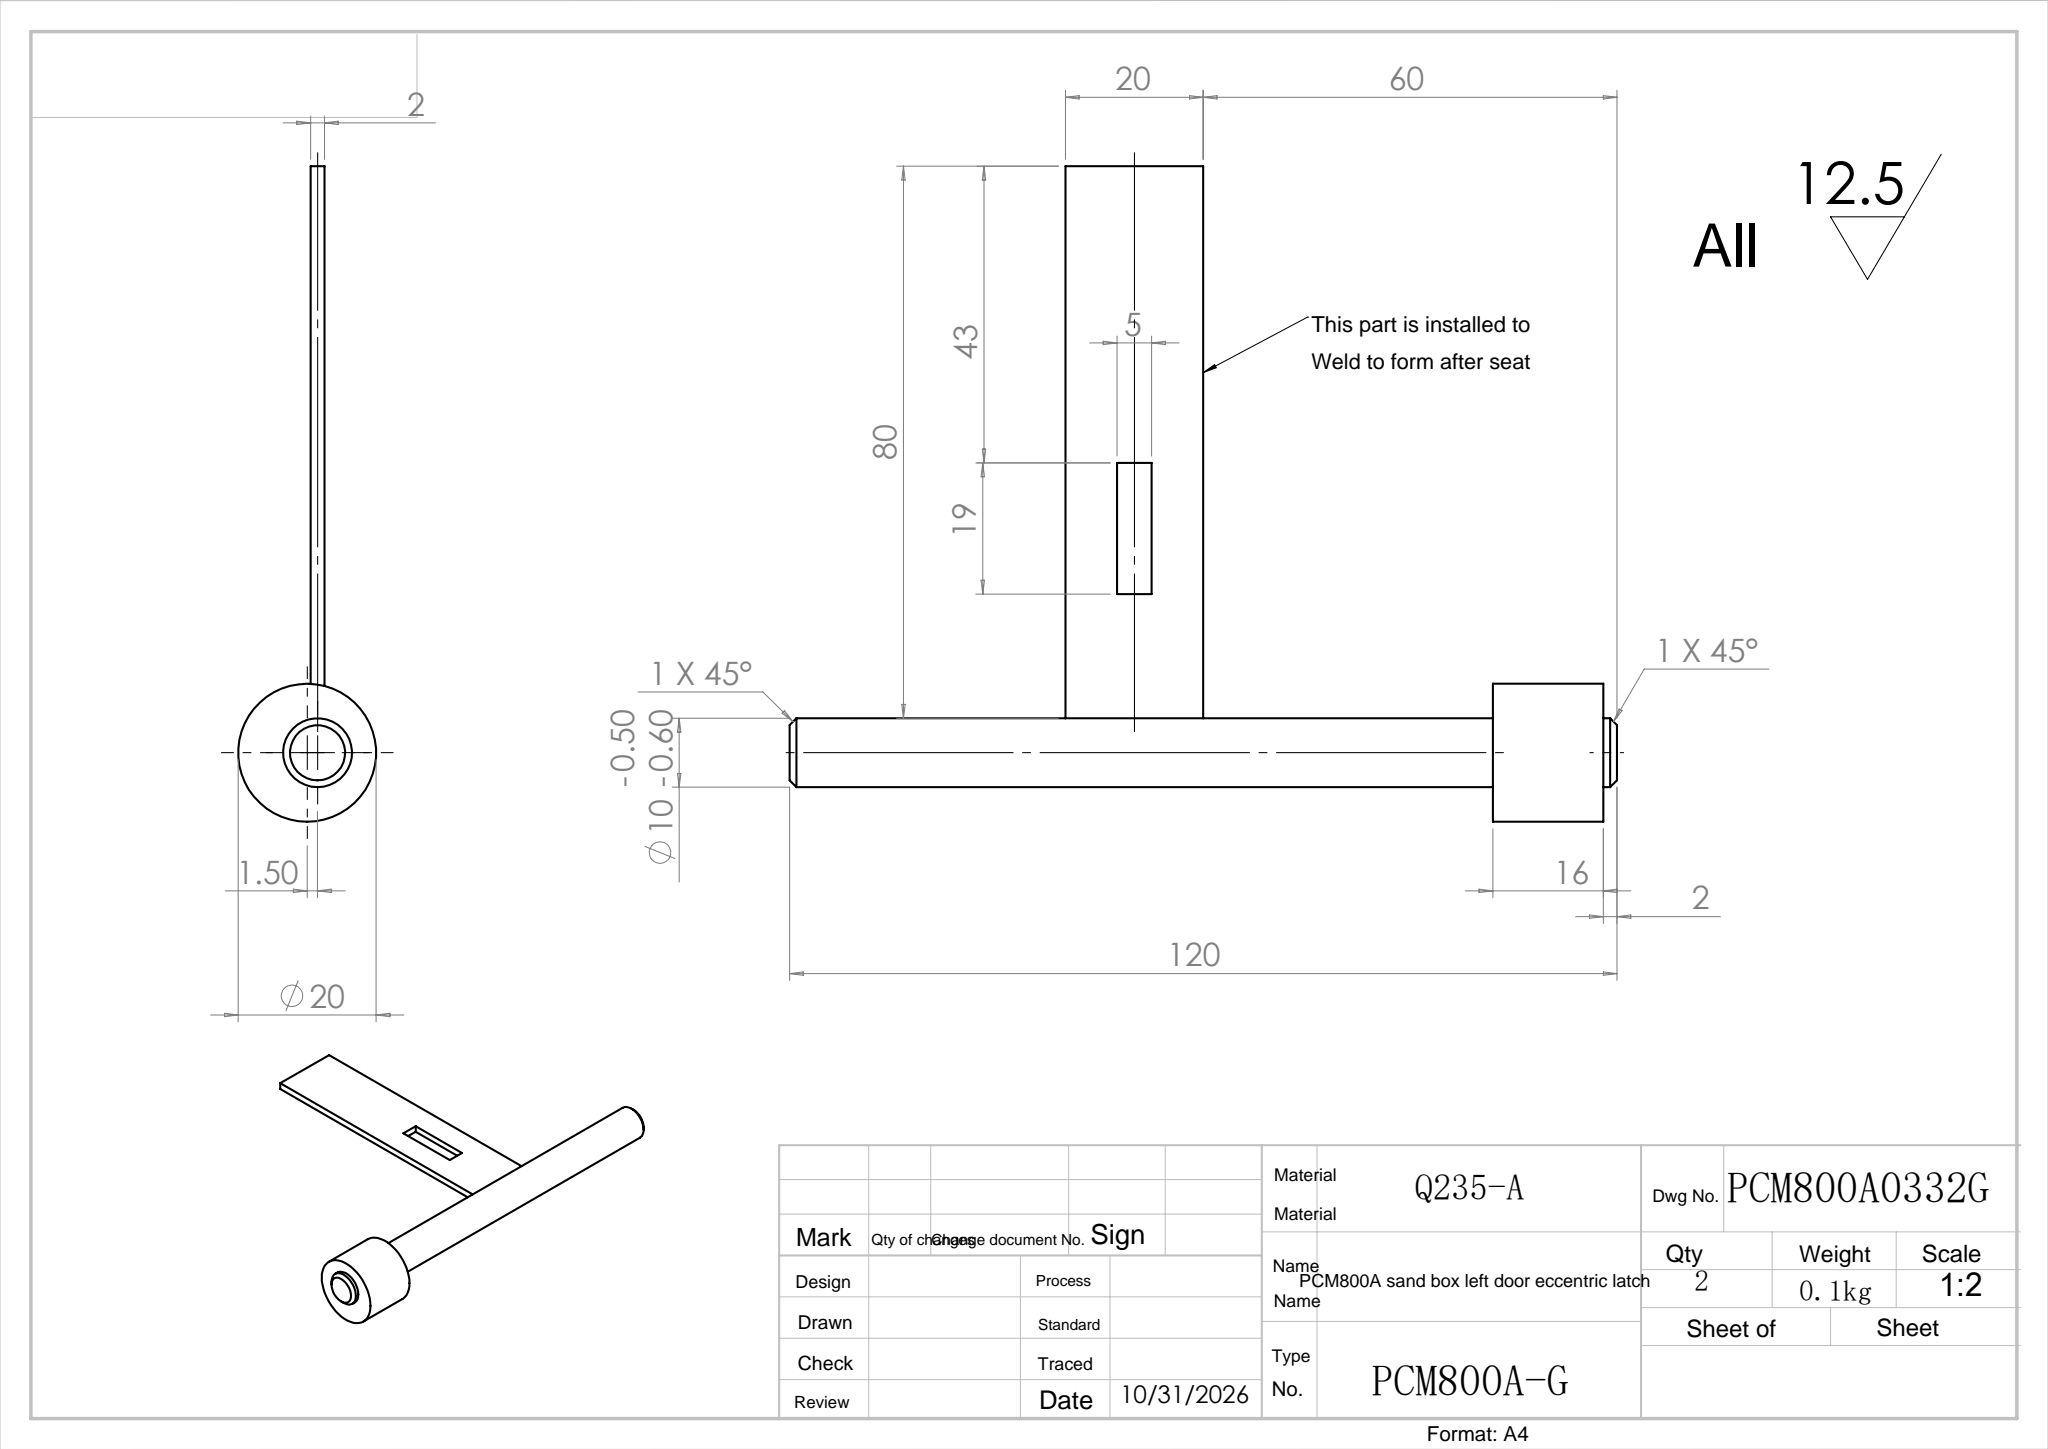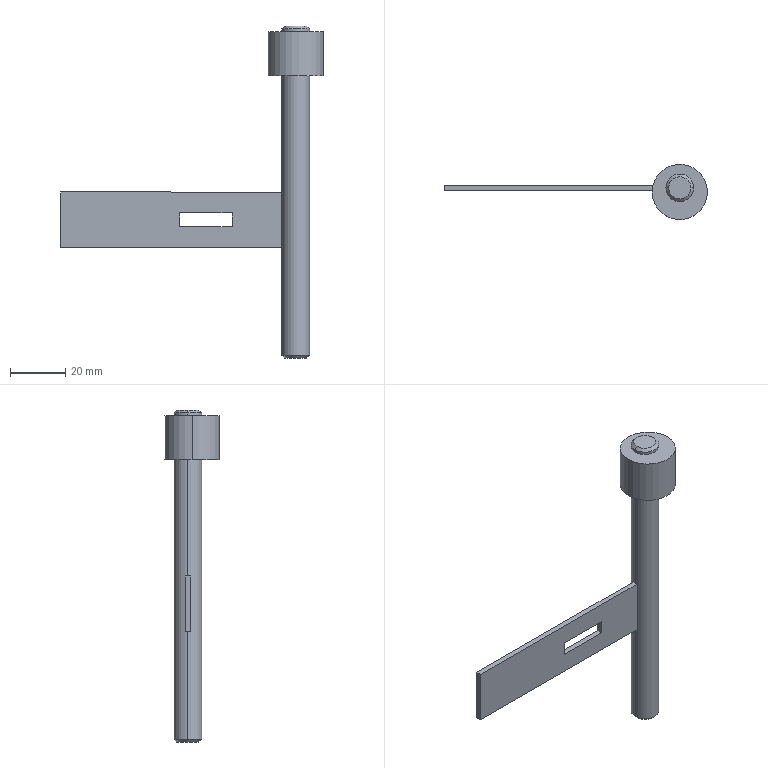Part | SolidWorks | features ICE 2, Chamfer 1, Extrusion 1 | 2 solids | 24 faces | box 95 x 20 x 120 mm | volume 16175 mm3 | plane 14 | cylinder 6 | cone 4 | commonest cylinder face diameters 10 x4 20 x2
STEP:
#1=CARTESIAN_POINT('',(4.,0.,120.));
#2=VERTEX_POINT('',#1);
#3=CARTESIAN_POINT('',(-4.,0.,120.));
#4=VERTEX_POINT('',#3);
#5=CARTESIAN_POINT('',(0.,0.,120.));
#6=DIRECTION('',(0.,0.,1.));
#7=DIRECTION('',(1.,0.,0.));
#8=AXIS2_PLACEMENT_3D('',#5,#6,#7);
#9=CIRCLE('',#8,4.);
#10=EDGE_CURVE('',#2,#4,#9,.T.);
#11=ORIENTED_EDGE('',*,*,#10,.F.);
#12=CARTESIAN_POINT('',(5.,0.,119.));
#13=VERTEX_POINT('',#12);
#14=CARTESIAN_POINT('',(4.,0.,120.));
#15=DIRECTION('',(0.7071,0.,-0.7071));
#16=VECTOR('',#15,1000.);
#17=LINE('',#14,#16);
#18=EDGE_CURVE('',#2,#13,#17,.T.);
#19=ORIENTED_EDGE('',*,*,#18,.T.);
#20=CARTESIAN_POINT('',(-5.,0.,119.));
#21=VERTEX_POINT('',#20);
#22=CARTESIAN_POINT('',(0.,0.,119.));
#23=DIRECTION('',(0.,0.,-1.));
#24=DIRECTION('',(1.,0.,0.));
#25=AXIS2_PLACEMENT_3D('',#22,#23,#24);
#26=CIRCLE('',#25,5.);
#27=EDGE_CURVE('',#21,#13,#26,.T.);
#28=ORIENTED_EDGE('',*,*,#27,.F.);
#29=CARTESIAN_POINT('',(-4.,0.,120.));
#30=DIRECTION('',(-0.7071,0.,-0.7071));
#31=VECTOR('',#30,1000.);
#32=LINE('',#29,#31);
#33=EDGE_CURVE('',#4,#21,#32,.T.);
#34=ORIENTED_EDGE('',*,*,#33,.F.);
#35=EDGE_LOOP('',(#11,#19,#28,#34));
#36=FACE_OUTER_BOUND('',#35,.T.);
#37=CARTESIAN_POINT('',(0.,0.,120.));
#38=DIRECTION('',(0.,0.,-1.));
#39=DIRECTION('',(-1.,0.,0.));
#40=AXIS2_PLACEMENT_3D('',#37,#38,#39);
#41=CONICAL_SURFACE('',#40,4.,0.7854);
#42=ADVANCED_FACE('',(#36),#41,.T.);
#43=CARTESIAN_POINT('',(-4.,0.,0.));
#44=VERTEX_POINT('',#43);
#45=CARTESIAN_POINT('',(4.,0.,0.));
#46=VERTEX_POINT('',#45);
#47=CARTESIAN_POINT('',(0.,0.,0.));
#48=DIRECTION('',(0.,0.,-1.));
#49=DIRECTION('',(1.,0.,0.));
#50=AXIS2_PLACEMENT_3D('',#47,#48,#49);
#51=CIRCLE('',#50,4.);
#52=EDGE_CURVE('',#44,#46,#51,.T.);
#53=ORIENTED_EDGE('',*,*,#52,.F.);
#54=CARTESIAN_POINT('',(-5.,0.,1.));
#55=VERTEX_POINT('',#54);
#56=CARTESIAN_POINT('',(-5.,0.,1.));
#57=DIRECTION('',(-0.7071,0.,0.7071));
#58=VECTOR('',#57,1000.);
#59=LINE('',#56,#58);
#60=EDGE_CURVE('',#44,#55,#59,.T.);
#61=ORIENTED_EDGE('',*,*,#60,.T.);
#62=CARTESIAN_POINT('',(5.,0.,1.));
#63=VERTEX_POINT('',#62);
#64=CARTESIAN_POINT('',(0.,0.,1.));
#65=DIRECTION('',(0.,0.,1.));
#66=DIRECTION('',(1.,0.,0.));
#67=AXIS2_PLACEMENT_3D('',#64,#65,#66);
#68=CIRCLE('',#67,5.);
#69=EDGE_CURVE('',#63,#55,#68,.T.);
#70=ORIENTED_EDGE('',*,*,#69,.F.);
#71=CARTESIAN_POINT('',(5.,0.,1.));
#72=DIRECTION('',(0.7071,0.,0.7071));
#73=VECTOR('',#72,1000.);
#74=LINE('',#71,#73);
#75=EDGE_CURVE('',#46,#63,#74,.T.);
#76=ORIENTED_EDGE('',*,*,#75,.F.);
#77=EDGE_LOOP('',(#53,#61,#70,#76));
#78=FACE_OUTER_BOUND('',#77,.T.);
#79=CARTESIAN_POINT('',(0.,0.,1.));
#80=DIRECTION('',(0.,0.,1.));
#81=DIRECTION('',(1.,0.,0.));
#82=AXIS2_PLACEMENT_3D('',#79,#80,#81);
#83=CONICAL_SURFACE('',#82,5.,0.7854);
#84=ADVANCED_FACE('',(#78),#83,.T.);
#85=ORIENTED_EDGE('',*,*,#27,.T.);
#86=CARTESIAN_POINT('',(5.,0.,118.));
#87=VERTEX_POINT('',#86);
#88=CARTESIAN_POINT('',(5.,0.,120.));
#89=DIRECTION('',(0.,0.,-1.));
#90=VECTOR('',#89,1000.);
#91=LINE('',#88,#90);
#92=EDGE_CURVE('',#13,#87,#91,.T.);
#93=ORIENTED_EDGE('',*,*,#92,.T.);
#94=CARTESIAN_POINT('',(-5.,0.,118.));
#95=VERTEX_POINT('',#94);
#96=CARTESIAN_POINT('',(0.,0.,118.));
#97=DIRECTION('',(0.,0.,1.));
#98=DIRECTION('',(1.,0.,0.));
#99=AXIS2_PLACEMENT_3D('',#96,#97,#98);
#100=CIRCLE('',#99,5.);
#101=EDGE_CURVE('',#87,#95,#100,.T.);
#102=ORIENTED_EDGE('',*,*,#101,.T.);
#103=CARTESIAN_POINT('',(-5.,0.,120.));
#104=DIRECTION('',(0.,0.,-1.));
#105=VECTOR('',#104,1000.);
#106=LINE('',#103,#105);
#107=EDGE_CURVE('',#21,#95,#106,.T.);
#108=ORIENTED_EDGE('',*,*,#107,.F.);
#109=EDGE_LOOP('',(#85,#93,#102,#108));
#110=FACE_OUTER_BOUND('',#109,.T.);
#111=CARTESIAN_POINT('',(0.,0.,120.));
#112=DIRECTION('',(0.,0.,-1.));
#113=DIRECTION('',(-1.,0.,0.));
#114=AXIS2_PLACEMENT_3D('',#111,#112,#113);
#115=CYLINDRICAL_SURFACE('',#114,5.);
#116=ADVANCED_FACE('',(#110),#115,.T.);
#117=CARTESIAN_POINT('',(10.,-1.5,102.));
#118=VERTEX_POINT('',#117);
#119=CARTESIAN_POINT('',(-10.,-1.5,102.));
#120=VERTEX_POINT('',#119);
#121=CARTESIAN_POINT('',(0.,-1.5,102.));
#122=DIRECTION('',(0.,0.,1.));
#123=DIRECTION('',(1.,0.,0.));
#124=AXIS2_PLACEMENT_3D('',#121,#122,#123);
#125=CIRCLE('',#124,10.);
#126=EDGE_CURVE('',#118,#120,#125,.T.);
#127=ORIENTED_EDGE('',*,*,#126,.T.);
#128=CARTESIAN_POINT('',(-10.,-1.5,118.));
#129=VERTEX_POINT('',#128);
#130=CARTESIAN_POINT('',(-10.,-1.5,102.));
#131=DIRECTION('',(0.,0.,1.));
#132=VECTOR('',#131,1000.);
#133=LINE('',#130,#132);
#134=EDGE_CURVE('',#120,#129,#133,.T.);
#135=ORIENTED_EDGE('',*,*,#134,.T.);
#136=CARTESIAN_POINT('',(10.,-1.5,118.));
#137=VERTEX_POINT('',#136);
#138=CARTESIAN_POINT('',(0.,-1.5,118.));
#139=DIRECTION('',(0.,0.,1.));
#140=DIRECTION('',(1.,0.,0.));
#141=AXIS2_PLACEMENT_3D('',#138,#139,#140);
#142=CIRCLE('',#141,10.);
#143=EDGE_CURVE('',#137,#129,#142,.T.);
#144=ORIENTED_EDGE('',*,*,#143,.F.);
#145=CARTESIAN_POINT('',(10.,-1.5,102.));
#146=DIRECTION('',(0.,0.,1.));
#147=VECTOR('',#146,1000.);
#148=LINE('',#145,#147);
#149=EDGE_CURVE('',#118,#137,#148,.T.);
#150=ORIENTED_EDGE('',*,*,#149,.F.);
#151=EDGE_LOOP('',(#127,#135,#144,#150));
#152=FACE_OUTER_BOUND('',#151,.T.);
#153=CARTESIAN_POINT('',(0.,-1.5,102.));
#154=DIRECTION('',(0.,0.,1.));
#155=DIRECTION('',(1.,0.,0.));
#156=AXIS2_PLACEMENT_3D('',#153,#154,#155);
#157=CYLINDRICAL_SURFACE('',#156,10.);
#158=ADVANCED_FACE('',(#152),#157,.T.);
#159=CARTESIAN_POINT('',(5.,0.,102.));
#160=VERTEX_POINT('',#159);
#161=CARTESIAN_POINT('',(-5.,0.,102.));
#162=VERTEX_POINT('',#161);
#163=CARTESIAN_POINT('',(0.,0.,102.));
#164=DIRECTION('',(0.,0.,1.));
#165=DIRECTION('',(1.,0.,0.));
#166=AXIS2_PLACEMENT_3D('',#163,#164,#165);
#167=CIRCLE('',#166,5.);
#168=EDGE_CURVE('',#160,#162,#167,.T.);
#169=ORIENTED_EDGE('',*,*,#168,.F.);
#170=CARTESIAN_POINT('',(5.,0.,120.));
#171=DIRECTION('',(0.,0.,-1.));
#172=VECTOR('',#171,1000.);
#173=LINE('',#170,#172);
#174=EDGE_CURVE('',#160,#63,#173,.T.);
#175=ORIENTED_EDGE('',*,*,#174,.T.);
#176=ORIENTED_EDGE('',*,*,#69,.T.);
#177=CARTESIAN_POINT('',(-5.,0.,120.));
#178=DIRECTION('',(0.,0.,-1.));
#179=VECTOR('',#178,1000.);
#180=LINE('',#177,#179);
#181=EDGE_CURVE('',#162,#55,#180,.T.);
#182=ORIENTED_EDGE('',*,*,#181,.F.);
#183=EDGE_LOOP('',(#169,#175,#176,#182));
#184=FACE_OUTER_BOUND('',#183,.T.);
#185=CARTESIAN_POINT('',(0.,0.,120.));
#186=DIRECTION('',(0.,0.,-1.));
#187=DIRECTION('',(-1.,0.,0.));
#188=AXIS2_PLACEMENT_3D('',#185,#186,#187);
#189=CYLINDRICAL_SURFACE('',#188,5.);
#190=ADVANCED_FACE('',(#184),#189,.T.);
#191=ORIENTED_EDGE('',*,*,#174,.F.);
#192=CARTESIAN_POINT('',(0.,0.,102.));
#193=DIRECTION('',(0.,0.,1.));
#194=DIRECTION('',(1.,0.,0.));
#195=AXIS2_PLACEMENT_3D('',#192,#193,#194);
#196=CIRCLE('',#195,5.);
#197=EDGE_CURVE('',#162,#160,#196,.T.);
#198=ORIENTED_EDGE('',*,*,#197,.F.);
#199=ORIENTED_EDGE('',*,*,#181,.T.);
#200=CARTESIAN_POINT('',(0.,0.,1.));
#201=DIRECTION('',(0.,0.,1.));
#202=DIRECTION('',(1.,0.,0.));
#203=AXIS2_PLACEMENT_3D('',#200,#201,#202);
#204=CIRCLE('',#203,5.);
#205=EDGE_CURVE('',#55,#63,#204,.T.);
#206=ORIENTED_EDGE('',*,*,#205,.T.);
#207=EDGE_LOOP('',(#191,#198,#199,#206));
#208=FACE_OUTER_BOUND('',#207,.T.);
#209=CARTESIAN_POINT('',(0.,0.,120.));
#210=DIRECTION('',(0.,0.,-1.));
#211=DIRECTION('',(-1.,0.,0.));
#212=AXIS2_PLACEMENT_3D('',#209,#210,#211);
#213=CYLINDRICAL_SURFACE('',#212,5.);
#214=ADVANCED_FACE('',(#208),#213,.T.);
#215=CARTESIAN_POINT('',(0.,0.,0.));
#216=DIRECTION('',(0.,0.,-1.));
#217=DIRECTION('',(1.,0.,0.));
#218=AXIS2_PLACEMENT_3D('',#215,#216,#217);
#219=CIRCLE('',#218,4.);
#220=EDGE_CURVE('',#46,#44,#219,.T.);
#221=ORIENTED_EDGE('',*,*,#220,.T.);
#222=ORIENTED_EDGE('',*,*,#52,.T.);
#223=EDGE_LOOP('',(#221,#222));
#224=FACE_OUTER_BOUND('',#223,.T.);
#225=CARTESIAN_POINT('',(0.,0.,0.));
#226=DIRECTION('',(0.,0.,1.));
#227=DIRECTION('',(1.,0.,0.));
#228=AXIS2_PLACEMENT_3D('',#225,#226,#227);
#229=PLANE('',#228);
#230=ADVANCED_FACE('',(#224),#229,.F.);
#231=ORIENTED_EDGE('',*,*,#126,.F.);
#232=CARTESIAN_POINT('',(0.,-1.5,102.));
#233=DIRECTION('',(0.,0.,1.));
#234=DIRECTION('',(1.,0.,0.));
#235=AXIS2_PLACEMENT_3D('',#232,#233,#234);
#236=CIRCLE('',#235,10.);
#237=EDGE_CURVE('',#120,#118,#236,.T.);
#238=ORIENTED_EDGE('',*,*,#237,.F.);
#239=EDGE_LOOP('',(#231,#238));
#240=FACE_OUTER_BOUND('',#239,.T.);
#241=ORIENTED_EDGE('',*,*,#197,.T.);
#242=ORIENTED_EDGE('',*,*,#168,.T.);
#243=EDGE_LOOP('',(#241,#242));
#244=FACE_BOUND('',#243,.T.);
#245=CARTESIAN_POINT('',(0.,-1.5,102.));
#246=DIRECTION('',(0.,0.,1.));
#247=DIRECTION('',(1.,0.,0.));
#248=AXIS2_PLACEMENT_3D('',#245,#246,#247);
#249=PLANE('',#248);
#250=ADVANCED_FACE('',(#240,#244),#249,.F.);
#251=ORIENTED_EDGE('',*,*,#143,.T.);
#252=CARTESIAN_POINT('',(0.,-1.5,118.));
#253=DIRECTION('',(0.,0.,1.));
#254=DIRECTION('',(1.,0.,0.));
#255=AXIS2_PLACEMENT_3D('',#252,#253,#254);
#256=CIRCLE('',#255,10.);
#257=EDGE_CURVE('',#129,#137,#256,.T.);
#258=ORIENTED_EDGE('',*,*,#257,.T.);
#259=EDGE_LOOP('',(#251,#258));
#260=FACE_OUTER_BOUND('',#259,.T.);
#261=CARTESIAN_POINT('',(0.,0.,118.));
#262=DIRECTION('',(0.,0.,1.));
#263=DIRECTION('',(1.,0.,0.));
#264=AXIS2_PLACEMENT_3D('',#261,#262,#263);
#265=CIRCLE('',#264,5.);
#266=EDGE_CURVE('',#95,#87,#265,.T.);
#267=ORIENTED_EDGE('',*,*,#266,.F.);
#268=ORIENTED_EDGE('',*,*,#101,.F.);
#269=EDGE_LOOP('',(#267,#268));
#270=FACE_BOUND('',#269,.T.);
#271=CARTESIAN_POINT('',(0.,-1.5,118.));
#272=DIRECTION('',(0.,0.,1.));
#273=DIRECTION('',(1.,0.,0.));
#274=AXIS2_PLACEMENT_3D('',#271,#272,#273);
#275=PLANE('',#274);
#276=ADVANCED_FACE('',(#260,#270),#275,.T.);
#277=ORIENTED_EDGE('',*,*,#134,.F.);
#278=ORIENTED_EDGE('',*,*,#237,.T.);
#279=ORIENTED_EDGE('',*,*,#149,.T.);
#280=ORIENTED_EDGE('',*,*,#257,.F.);
#281=EDGE_LOOP('',(#277,#278,#279,#280));
#282=FACE_OUTER_BOUND('',#281,.T.);
#283=CARTESIAN_POINT('',(0.,-1.5,102.));
#284=DIRECTION('',(0.,0.,1.));
#285=DIRECTION('',(1.,0.,0.));
#286=AXIS2_PLACEMENT_3D('',#283,#284,#285);
#287=CYLINDRICAL_SURFACE('',#286,10.);
#288=ADVANCED_FACE('',(#282),#287,.T.);
#289=CARTESIAN_POINT('',(0.,0.,120.));
#290=DIRECTION('',(0.,0.,1.));
#291=DIRECTION('',(1.,0.,0.));
#292=AXIS2_PLACEMENT_3D('',#289,#290,#291);
#293=CIRCLE('',#292,4.);
#294=EDGE_CURVE('',#4,#2,#293,.T.);
#295=ORIENTED_EDGE('',*,*,#294,.T.);
#296=ORIENTED_EDGE('',*,*,#10,.T.);
#297=EDGE_LOOP('',(#295,#296));
#298=FACE_OUTER_BOUND('',#297,.T.);
#299=CARTESIAN_POINT('',(0.,0.,120.));
#300=DIRECTION('',(0.,0.,1.));
#301=DIRECTION('',(1.,0.,0.));
#302=AXIS2_PLACEMENT_3D('',#299,#300,#301);
#303=PLANE('',#302);
#304=ADVANCED_FACE('',(#298),#303,.T.);
#305=ORIENTED_EDGE('',*,*,#92,.F.);
#306=CARTESIAN_POINT('',(0.,0.,119.));
#307=DIRECTION('',(0.,0.,-1.));
#308=DIRECTION('',(1.,0.,0.));
#309=AXIS2_PLACEMENT_3D('',#306,#307,#308);
#310=CIRCLE('',#309,5.);
#311=EDGE_CURVE('',#13,#21,#310,.T.);
#312=ORIENTED_EDGE('',*,*,#311,.T.);
#313=ORIENTED_EDGE('',*,*,#107,.T.);
#314=ORIENTED_EDGE('',*,*,#266,.T.);
#315=EDGE_LOOP('',(#305,#312,#313,#314));
#316=FACE_OUTER_BOUND('',#315,.T.);
#317=CARTESIAN_POINT('',(0.,0.,120.));
#318=DIRECTION('',(0.,0.,-1.));
#319=DIRECTION('',(-1.,0.,0.));
#320=AXIS2_PLACEMENT_3D('',#317,#318,#319);
#321=CYLINDRICAL_SURFACE('',#320,5.);
#322=ADVANCED_FACE('',(#316),#321,.T.);
#323=ORIENTED_EDGE('',*,*,#60,.F.);
#324=ORIENTED_EDGE('',*,*,#220,.F.);
#325=ORIENTED_EDGE('',*,*,#75,.T.);
#326=ORIENTED_EDGE('',*,*,#205,.F.);
#327=EDGE_LOOP('',(#323,#324,#325,#326));
#328=FACE_OUTER_BOUND('',#327,.T.);
#329=CARTESIAN_POINT('',(0.,0.,1.));
#330=DIRECTION('',(0.,0.,1.));
#331=DIRECTION('',(1.,0.,0.));
#332=AXIS2_PLACEMENT_3D('',#329,#330,#331);
#333=CONICAL_SURFACE('',#332,5.,0.7854);
#334=ADVANCED_FACE('',(#328),#333,.T.);
#335=ORIENTED_EDGE('',*,*,#18,.F.);
#336=ORIENTED_EDGE('',*,*,#294,.F.);
#337=ORIENTED_EDGE('',*,*,#33,.T.);
#338=ORIENTED_EDGE('',*,*,#311,.F.);
#339=EDGE_LOOP('',(#335,#336,#337,#338));
#340=FACE_OUTER_BOUND('',#339,.T.);
#341=CARTESIAN_POINT('',(0.,0.,120.));
#342=DIRECTION('',(0.,0.,-1.));
#343=DIRECTION('',(-1.,0.,0.));
#344=AXIS2_PLACEMENT_3D('',#341,#342,#343);
#345=CONICAL_SURFACE('',#344,4.,0.7854);
#346=ADVANCED_FACE('',(#340),#345,.T.);
#347=CLOSED_SHELL('',(#42,#84,#116,#158,#190,#214,#230,#250,#276,#288,#304,#322,#334,#346));
#348=MANIFOLD_SOLID_BREP('',#347);
#349=CARTESIAN_POINT('',(-5.,1.,60.));
#350=VERTEX_POINT('',#349);
#351=CARTESIAN_POINT('',(-5.,1.,40.));
#352=VERTEX_POINT('',#351);
#353=CARTESIAN_POINT('',(-5.,1.,40.));
#354=DIRECTION('',(0.,0.,-1.));
#355=VECTOR('',#354,1000.);
#356=LINE('',#353,#355);
#357=EDGE_CURVE('',#350,#352,#356,.T.);
#358=ORIENTED_EDGE('',*,*,#357,.T.);
#359=CARTESIAN_POINT('',(-85.,1.,40.));
#360=VERTEX_POINT('',#359);
#361=CARTESIAN_POINT('',(-5.,1.,40.));
#362=DIRECTION('',(-1.,0.,0.));
#363=VECTOR('',#362,1000.);
#364=LINE('',#361,#363);
#365=EDGE_CURVE('',#352,#360,#364,.T.);
#366=ORIENTED_EDGE('',*,*,#365,.T.);
#367=CARTESIAN_POINT('',(-85.,1.,60.));
#368=VERTEX_POINT('',#367);
#369=CARTESIAN_POINT('',(-85.,1.,40.));
#370=DIRECTION('',(0.,0.,1.));
#371=VECTOR('',#370,1000.);
#372=LINE('',#369,#371);
#373=EDGE_CURVE('',#360,#368,#372,.T.);
#374=ORIENTED_EDGE('',*,*,#373,.T.);
#375=CARTESIAN_POINT('',(-5.,1.,60.));
#376=DIRECTION('',(1.,0.,0.));
#377=VECTOR('',#376,1000.);
#378=LINE('',#375,#377);
#379=EDGE_CURVE('',#368,#350,#378,.T.);
#380=ORIENTED_EDGE('',*,*,#379,.T.);
#381=EDGE_LOOP('',(#358,#366,#374,#380));
#382=FACE_OUTER_BOUND('',#381,.T.);
#383=CARTESIAN_POINT('',(-42.,1.,47.5));
#384=VERTEX_POINT('',#383);
#385=CARTESIAN_POINT('',(-42.,1.,52.5));
#386=VERTEX_POINT('',#385);
#387=CARTESIAN_POINT('',(-42.,1.,47.5));
#388=DIRECTION('',(0.,0.,1.));
#389=VECTOR('',#388,1000.);
#390=LINE('',#387,#389);
#391=EDGE_CURVE('',#384,#386,#390,.T.);
#392=ORIENTED_EDGE('',*,*,#391,.F.);
#393=CARTESIAN_POINT('',(-23.,1.,47.5));
#394=VERTEX_POINT('',#393);
#395=CARTESIAN_POINT('',(-42.,1.,47.5));
#396=DIRECTION('',(-1.,0.,0.));
#397=VECTOR('',#396,1000.);
#398=LINE('',#395,#397);
#399=EDGE_CURVE('',#394,#384,#398,.T.);
#400=ORIENTED_EDGE('',*,*,#399,.F.);
#401=CARTESIAN_POINT('',(-23.,1.,52.5));
#402=VERTEX_POINT('',#401);
#403=CARTESIAN_POINT('',(-23.,1.,47.5));
#404=DIRECTION('',(0.,0.,-1.));
#405=VECTOR('',#404,1000.);
#406=LINE('',#403,#405);
#407=EDGE_CURVE('',#402,#394,#406,.T.);
#408=ORIENTED_EDGE('',*,*,#407,.F.);
#409=CARTESIAN_POINT('',(-42.,1.,52.5));
#410=DIRECTION('',(1.,0.,0.));
#411=VECTOR('',#410,1000.);
#412=LINE('',#409,#411);
#413=EDGE_CURVE('',#386,#402,#412,.T.);
#414=ORIENTED_EDGE('',*,*,#413,.F.);
#415=EDGE_LOOP('',(#392,#400,#408,#414));
#416=FACE_BOUND('',#415,.T.);
#417=CARTESIAN_POINT('',(-5.,1.,60.));
#418=DIRECTION('',(0.,-1.,0.));
#419=DIRECTION('',(0.,0.,-1.));
#420=AXIS2_PLACEMENT_3D('',#417,#418,#419);
#421=PLANE('',#420);
#422=ADVANCED_FACE('',(#382,#416),#421,.F.);
#423=CARTESIAN_POINT('',(-5.,-1.,60.));
#424=VERTEX_POINT('',#423);
#425=CARTESIAN_POINT('',(-5.,-1.,40.));
#426=VERTEX_POINT('',#425);
#427=CARTESIAN_POINT('',(-5.,-1.,40.));
#428=DIRECTION('',(0.,0.,-1.));
#429=VECTOR('',#428,1000.);
#430=LINE('',#427,#429);
#431=EDGE_CURVE('',#424,#426,#430,.T.);
#432=ORIENTED_EDGE('',*,*,#431,.F.);
#433=CARTESIAN_POINT('',(-85.,-1.,60.));
#434=VERTEX_POINT('',#433);
#435=CARTESIAN_POINT('',(-5.,-1.,60.));
#436=DIRECTION('',(1.,0.,0.));
#437=VECTOR('',#436,1000.);
#438=LINE('',#435,#437);
#439=EDGE_CURVE('',#434,#424,#438,.T.);
#440=ORIENTED_EDGE('',*,*,#439,.F.);
#441=CARTESIAN_POINT('',(-85.,-1.,40.));
#442=VERTEX_POINT('',#441);
#443=CARTESIAN_POINT('',(-85.,-1.,40.));
#444=DIRECTION('',(0.,0.,1.));
#445=VECTOR('',#444,1000.);
#446=LINE('',#443,#445);
#447=EDGE_CURVE('',#442,#434,#446,.T.);
#448=ORIENTED_EDGE('',*,*,#447,.F.);
#449=CARTESIAN_POINT('',(-5.,-1.,40.));
#450=DIRECTION('',(-1.,0.,0.));
#451=VECTOR('',#450,1000.);
#452=LINE('',#449,#451);
#453=EDGE_CURVE('',#426,#442,#452,.T.);
#454=ORIENTED_EDGE('',*,*,#453,.F.);
#455=EDGE_LOOP('',(#432,#440,#448,#454));
#456=FACE_OUTER_BOUND('',#455,.T.);
#457=CARTESIAN_POINT('',(-23.,-1.,47.5));
#458=VERTEX_POINT('',#457);
#459=CARTESIAN_POINT('',(-42.,-1.,47.5));
#460=VERTEX_POINT('',#459);
#461=CARTESIAN_POINT('',(-42.,-1.,47.5));
#462=DIRECTION('',(-1.,0.,0.));
#463=VECTOR('',#462,1000.);
#464=LINE('',#461,#463);
#465=EDGE_CURVE('',#458,#460,#464,.T.);
#466=ORIENTED_EDGE('',*,*,#465,.T.);
#467=CARTESIAN_POINT('',(-42.,-1.,52.5));
#468=VERTEX_POINT('',#467);
#469=CARTESIAN_POINT('',(-42.,-1.,47.5));
#470=DIRECTION('',(0.,0.,1.));
#471=VECTOR('',#470,1000.);
#472=LINE('',#469,#471);
#473=EDGE_CURVE('',#460,#468,#472,.T.);
#474=ORIENTED_EDGE('',*,*,#473,.T.);
#475=CARTESIAN_POINT('',(-23.,-1.,52.5));
#476=VERTEX_POINT('',#475);
#477=CARTESIAN_POINT('',(-42.,-1.,52.5));
#478=DIRECTION('',(1.,0.,0.));
#479=VECTOR('',#478,1000.);
#480=LINE('',#477,#479);
#481=EDGE_CURVE('',#468,#476,#480,.T.);
#482=ORIENTED_EDGE('',*,*,#481,.T.);
#483=CARTESIAN_POINT('',(-23.,-1.,47.5));
#484=DIRECTION('',(0.,0.,-1.));
#485=VECTOR('',#484,1000.);
#486=LINE('',#483,#485);
#487=EDGE_CURVE('',#476,#458,#486,.T.);
#488=ORIENTED_EDGE('',*,*,#487,.T.);
#489=EDGE_LOOP('',(#466,#474,#482,#488));
#490=FACE_BOUND('',#489,.T.);
#491=CARTESIAN_POINT('',(-5.,-1.,60.));
#492=DIRECTION('',(0.,-1.,0.));
#493=DIRECTION('',(0.,0.,-1.));
#494=AXIS2_PLACEMENT_3D('',#491,#492,#493);
#495=PLANE('',#494);
#496=ADVANCED_FACE('',(#456,#490),#495,.T.);
#497=ORIENTED_EDGE('',*,*,#431,.T.);
#498=CARTESIAN_POINT('',(-5.,1.,40.));
#499=DIRECTION('',(0.,-1.,0.));
#500=VECTOR('',#499,1000.);
#501=LINE('',#498,#500);
#502=EDGE_CURVE('',#352,#426,#501,.T.);
#503=ORIENTED_EDGE('',*,*,#502,.F.);
#504=ORIENTED_EDGE('',*,*,#357,.F.);
#505=CARTESIAN_POINT('',(-5.,1.,60.));
#506=DIRECTION('',(0.,-1.,0.));
#507=VECTOR('',#506,1000.);
#508=LINE('',#505,#507);
#509=EDGE_CURVE('',#350,#424,#508,.T.);
#510=ORIENTED_EDGE('',*,*,#509,.T.);
#511=EDGE_LOOP('',(#497,#503,#504,#510));
#512=FACE_OUTER_BOUND('',#511,.T.);
#513=CARTESIAN_POINT('',(-5.,1.,40.));
#514=DIRECTION('',(-1.,0.,0.));
#515=DIRECTION('',(0.,0.,1.));
#516=AXIS2_PLACEMENT_3D('',#513,#514,#515);
#517=PLANE('',#516);
#518=ADVANCED_FACE('',(#512),#517,.F.);
#519=ORIENTED_EDGE('',*,*,#453,.T.);
#520=CARTESIAN_POINT('',(-85.,1.,40.));
#521=DIRECTION('',(0.,-1.,0.));
#522=VECTOR('',#521,1000.);
#523=LINE('',#520,#522);
#524=EDGE_CURVE('',#360,#442,#523,.T.);
#525=ORIENTED_EDGE('',*,*,#524,.F.);
#526=ORIENTED_EDGE('',*,*,#365,.F.);
#527=ORIENTED_EDGE('',*,*,#502,.T.);
#528=EDGE_LOOP('',(#519,#525,#526,#527));
#529=FACE_OUTER_BOUND('',#528,.T.);
#530=CARTESIAN_POINT('',(-5.,1.,40.));
#531=DIRECTION('',(0.,0.,1.));
#532=DIRECTION('',(1.,0.,0.));
#533=AXIS2_PLACEMENT_3D('',#530,#531,#532);
#534=PLANE('',#533);
#535=ADVANCED_FACE('',(#529),#534,.F.);
#536=ORIENTED_EDGE('',*,*,#447,.T.);
#537=CARTESIAN_POINT('',(-85.,1.,60.));
#538=DIRECTION('',(0.,-1.,0.));
#539=VECTOR('',#538,1000.);
#540=LINE('',#537,#539);
#541=EDGE_CURVE('',#368,#434,#540,.T.);
#542=ORIENTED_EDGE('',*,*,#541,.F.);
#543=ORIENTED_EDGE('',*,*,#373,.F.);
#544=ORIENTED_EDGE('',*,*,#524,.T.);
#545=EDGE_LOOP('',(#536,#542,#543,#544));
#546=FACE_OUTER_BOUND('',#545,.T.);
#547=CARTESIAN_POINT('',(-85.,1.,40.));
#548=DIRECTION('',(1.,0.,0.));
#549=DIRECTION('',(0.,0.,-1.));
#550=AXIS2_PLACEMENT_3D('',#547,#548,#549);
#551=PLANE('',#550);
#552=ADVANCED_FACE('',(#546),#551,.F.);
#553=ORIENTED_EDGE('',*,*,#439,.T.);
#554=ORIENTED_EDGE('',*,*,#509,.F.);
#555=ORIENTED_EDGE('',*,*,#379,.F.);
#556=ORIENTED_EDGE('',*,*,#541,.T.);
#557=EDGE_LOOP('',(#553,#554,#555,#556));
#558=FACE_OUTER_BOUND('',#557,.T.);
#559=CARTESIAN_POINT('',(-5.,1.,60.));
#560=DIRECTION('',(0.,0.,-1.));
#561=DIRECTION('',(-1.,0.,0.));
#562=AXIS2_PLACEMENT_3D('',#559,#560,#561);
#563=PLANE('',#562);
#564=ADVANCED_FACE('',(#558),#563,.F.);
#565=ORIENTED_EDGE('',*,*,#473,.F.);
#566=CARTESIAN_POINT('',(-42.,1.,47.5));
#567=DIRECTION('',(0.,-1.,0.));
#568=VECTOR('',#567,1000.);
#569=LINE('',#566,#568);
#570=EDGE_CURVE('',#384,#460,#569,.T.);
#571=ORIENTED_EDGE('',*,*,#570,.F.);
#572=ORIENTED_EDGE('',*,*,#391,.T.);
#573=CARTESIAN_POINT('',(-42.,1.,52.5));
#574=DIRECTION('',(0.,-1.,0.));
#575=VECTOR('',#574,1000.);
#576=LINE('',#573,#575);
#577=EDGE_CURVE('',#386,#468,#576,.T.);
#578=ORIENTED_EDGE('',*,*,#577,.T.);
#579=EDGE_LOOP('',(#565,#571,#572,#578));
#580=FACE_OUTER_BOUND('',#579,.T.);
#581=CARTESIAN_POINT('',(-42.,1.,47.5));
#582=DIRECTION('',(1.,0.,0.));
#583=DIRECTION('',(0.,0.,-1.));
#584=AXIS2_PLACEMENT_3D('',#581,#582,#583);
#585=PLANE('',#584);
#586=ADVANCED_FACE('',(#580),#585,.T.);
#587=ORIENTED_EDGE('',*,*,#481,.F.);
#588=ORIENTED_EDGE('',*,*,#577,.F.);
#589=ORIENTED_EDGE('',*,*,#413,.T.);
#590=CARTESIAN_POINT('',(-23.,1.,52.5));
#591=DIRECTION('',(0.,-1.,0.));
#592=VECTOR('',#591,1000.);
#593=LINE('',#590,#592);
#594=EDGE_CURVE('',#402,#476,#593,.T.);
#595=ORIENTED_EDGE('',*,*,#594,.T.);
#596=EDGE_LOOP('',(#587,#588,#589,#595));
#597=FACE_OUTER_BOUND('',#596,.T.);
#598=CARTESIAN_POINT('',(-42.,1.,52.5));
#599=DIRECTION('',(0.,0.,-1.));
#600=DIRECTION('',(-1.,0.,0.));
#601=AXIS2_PLACEMENT_3D('',#598,#599,#600);
#602=PLANE('',#601);
#603=ADVANCED_FACE('',(#597),#602,.T.);
#604=ORIENTED_EDGE('',*,*,#487,.F.);
#605=ORIENTED_EDGE('',*,*,#594,.F.);
#606=ORIENTED_EDGE('',*,*,#407,.T.);
#607=CARTESIAN_POINT('',(-23.,1.,47.5));
#608=DIRECTION('',(0.,-1.,0.));
#609=VECTOR('',#608,1000.);
#610=LINE('',#607,#609);
#611=EDGE_CURVE('',#394,#458,#610,.T.);
#612=ORIENTED_EDGE('',*,*,#611,.T.);
#613=EDGE_LOOP('',(#604,#605,#606,#612));
#614=FACE_OUTER_BOUND('',#613,.T.);
#615=CARTESIAN_POINT('',(-23.,1.,47.5));
#616=DIRECTION('',(-1.,0.,0.));
#617=DIRECTION('',(0.,0.,1.));
#618=AXIS2_PLACEMENT_3D('',#615,#616,#617);
#619=PLANE('',#618);
#620=ADVANCED_FACE('',(#614),#619,.T.);
#621=ORIENTED_EDGE('',*,*,#465,.F.);
#622=ORIENTED_EDGE('',*,*,#611,.F.);
#623=ORIENTED_EDGE('',*,*,#399,.T.);
#624=ORIENTED_EDGE('',*,*,#570,.T.);
#625=EDGE_LOOP('',(#621,#622,#623,#624));
#626=FACE_OUTER_BOUND('',#625,.T.);
#627=CARTESIAN_POINT('',(-42.,1.,47.5));
#628=DIRECTION('',(0.,0.,1.));
#629=DIRECTION('',(1.,0.,0.));
#630=AXIS2_PLACEMENT_3D('',#627,#628,#629);
#631=PLANE('',#630);
#632=ADVANCED_FACE('',(#626),#631,.T.);
#633=CLOSED_SHELL('',(#422,#496,#518,#535,#552,#564,#586,#603,#620,#632));
#634=MANIFOLD_SOLID_BREP('',#633);
#635=CARTESIAN_POINT('',(0.,0.,0.));
#636=DIRECTION('',(0.,0.,1.));
#637=DIRECTION('',(1.,0.,0.));
#638=AXIS2_PLACEMENT_3D('',#635,#636,#637);
#639=(LENGTH_UNIT()NAMED_UNIT(*)SI_UNIT(.MILLI.,.METRE.));
#640=UNCERTAINTY_MEASURE_WITH_UNIT(LENGTH_MEASURE(0.00001),#639,'','');
#641=(NAMED_UNIT(*)PLANE_ANGLE_UNIT()SI_UNIT($,.RADIAN.));
#642=(NAMED_UNIT(*)SI_UNIT($,.STERADIAN.)SOLID_ANGLE_UNIT());
#643=(GEOMETRIC_REPRESENTATION_CONTEXT(3)GLOBAL_UNCERTAINTY_ASSIGNED_CONTEXT((#640))GLOBAL_UNIT_ASSIGNED_CONTEXT((#639,#641,#642))REPRESENTATION_CONTEXT('',''));
#644=ADVANCED_BREP_SHAPE_REPRESENTATION('',(#348,#634,#638),#643);